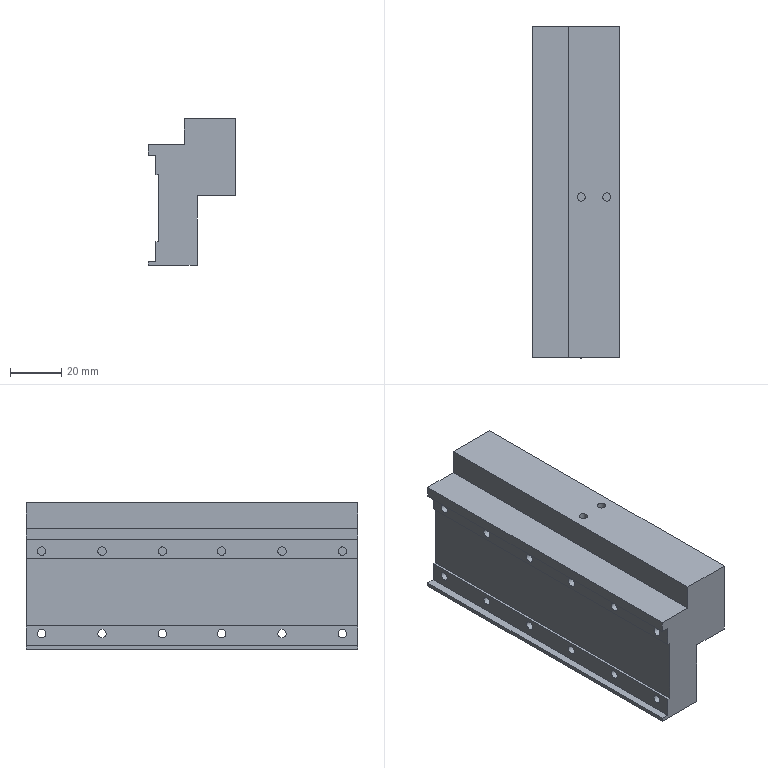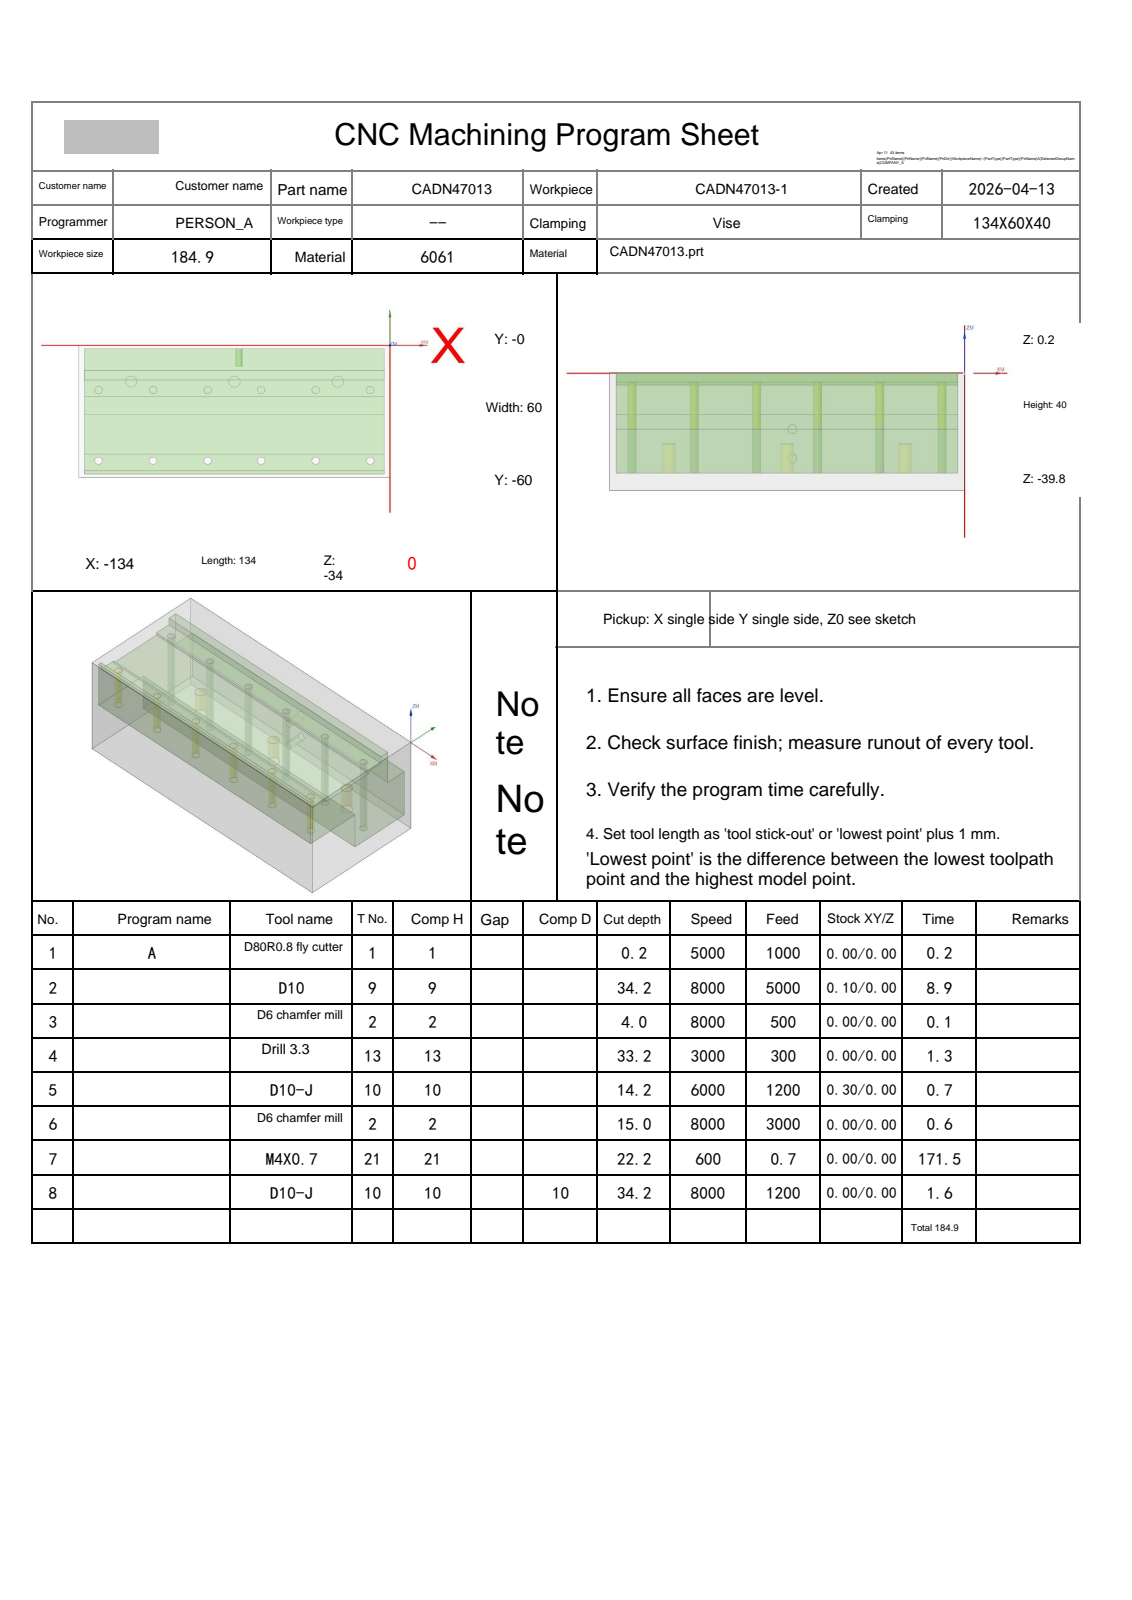NC program | NX | posted by the shop | part box 34 x 129 x 57 mm
Whole program:
%
O0001
(Machine time: 349.26 MIN)
(===Total Tool:6===)
(T1=D80R0.8 fly cutter D=80.  R=0.8  D-  H01 Z=-0.   )
(T9=D10     D=10.  R=0.   D-  H09 Z=-34.  )
(T2=D6 chamfer mill   D=6.   R=0.   D-  H02 Z=-14.8 )
(T13=Drill 3.3  D=3.3  DR_a=118 D-  H13 Z=-33.  )
(T10=D10-J  D=10.  R=0.   D-  H10 Z=-34.  )
(T21=M4X0.7 D=3.3  DR_a=180 D-  H21 Z=-22.  )
G80 G90 G17 G49 G40
G91 G28 Z0
M01
N1 T01 M06
(D80R0.8 fly cutter  D=80. R=0.8 H=01 ce=0.00 di=0.00)
G00 G90 G54 X42.5 Y-30. M03 S5000
G43 H01 Z20.
M08
Z2.
G01 Z0.0 F1000.
X37.5
X-171.5
X-176.5
Z2.
G00 Z20.
G91 G28 Z0.0
M05
M09
G91 G28 Z0.0
M01
N2 T09 M06
(D10  D=10. R=0. H=09 ce=0.10 di=0.00)
G00 G90 G54 X-67. Y3.6 M03 S8000
G43 H09 Z20.
M08
Z.5
G01 X-2.5 Z.375 F5000.
G02 X2.6 Y-1.5 Z.359 I0.0 J-5.1
G01 Y-58.5 Z.249
G02 X-2.5 Y-63.6 Z.233 I-5.1 J0.0
G01 X-131.5 Z-.017
G02 X-136.6 Y-58.5 Z-.033 I0.0 J5.1
G01 Y-1.5 Z-.143
G02 X-131.5 Y3.6 Z-.159 I5.1 J0.0
G01 X-2.5 Z-.409
G02 X2.6 Y-1.5 Z-.425 I0.0 J-5.1
G01 Y-58.5 Z-.535
G02 X-2.5 Y-63.6 Z-.551 I-5.1 J0.0
G01 X-131.5 Z-.801
G02 X-136.6 Y-58.5 Z-.817 I0.0 J5.1
G01 Y-1.5 Z-.927
G02 X-131.5 Y3.6 Z-.943 I5.1 J0.0
G01 X-2.5 Z-1.193
G02 X2.6 Y-1.5 Z-1.209 I0.0 J-5.1
G01 Y-58.5 Z-1.32
G02 X-2.5 Y-63.6 Z-1.335 I-5.1 J0.0
G01 X-131.5 Z-1.585
G02 X-136.6 Y-58.5 Z-1.601 I0.0 J5.1
G01 Y-1.5 Z-1.712
G02 X-131.5 Y3.6 Z-1.727 I5.1 J0.0
G01 X-2.5 Z-1.977
G02 X2.6 Y-1.5 Z-1.993 I0.0 J-5.1
G01 Y-58.5 Z-2.104
G02 X-2.5 Y-63.6 Z-2.119 I-5.1 J0.0
G01 X-131.5 Z-2.369
G02 X-136.6 Y-58.5 Z-2.385 I0.0 J5.1
G01 Y-1.5 Z-2.496
G02 X-131.5 Y3.6 Z-2.511 I5.1 J0.0
G01 X-2.5 Z-2.762
G02 X2.6 Y-1.5 Z-2.777 I0.0 J-5.1
G01 Y-58.5 Z-2.888
G02 X-2.5 Y-63.6 Z-2.903 I-5.1 J0.0
G01 X-131.5 Z-3.154
G02 X-136.6 Y-58.5 Z-3.169 I0.0 J5.1
G01 Y-1.5 Z-3.28
G02 X-131.5 Y3.6 Z-3.295 I5.1 J0.0
G01 X-2.5 Z-3.546
G02 X2.6 Y-1.5 Z-3.561 I0.0 J-5.1
G01 Y-58.5 Z-3.672
G02 X-2.5 Y-63.6 Z-3.687 I-5.1 J0.0
G01 X-131.5 Z-3.938
G02 X-136.6 Y-58.5 Z-3.953 I0.0 J5.1
G01 Y-1.5 Z-4.064
G02 X-131.5 Y3.6 Z-4.079 I5.1 J0.0
G01 X-2.5 Z-4.33
G02 X2.6 Y-1.5 Z-4.345 I0.0 J-5.1
G01 Y-58.5 Z-4.456
G02 X-2.5 Y-63.6 Z-4.471 I-5.1 J0.0
G01 X-131.5 Z-4.722
G02 X-136.6 Y-58.5 Z-4.737 I0.0 J5.1
G01 Y-1.5 Z-4.848
G02 X-131.5 Y3.6 Z-4.863 I5.1 J0.0
G01 X-2.5 Z-5.114
G02 X2.6 Y-1.5 Z-5.129 I0.0 J-5.1
G01 Y-58.5 Z-5.24
G02 X-2.5 Y-63.6 Z-5.256 I-5.1 J0.0
G01 X-131.5 Z-5.506
G02 X-136.6 Y-58.5 Z-5.521 I0.0 J5.1
G01 Y-1.5 Z-5.632
G02 X-131.5 Y3.6 Z-5.648 I5.1 J0.0
G01 X-2.5 Z-5.898
G02 X2.6 Y-1.5 Z-5.913 I0.0 J-5.1
G01 Y-58.5 Z-6.024
G02 X-2.5 Y-63.6 Z-6.04 I-5.1 J0.0
G01 X-131.5 Z-6.29
G02 X-136.6 Y-58.5 Z-6.305 I0.0 J5.1
G01 Y-1.5 Z-6.416
G02 X-131.5 Y3.6 Z-6.432 I5.1 J0.0
G01 X-2.5 Z-6.682
G02 X2.6 Y-1.5 Z-6.698 I0.0 J-5.1
G01 Y-58.5 Z-6.808
G02 X-2.5 Y-63.6 Z-6.824 I-5.1 J0.0
G01 X-131.5 Z-7.074
G02 X-136.6 Y-58.5 Z-7.09 I0.0 J5.1
G01 Y-1.5 Z-7.2
G02 X-131.5 Y3.6 Z-7.216 I5.1 J0.0
G01 X-2.5 Z-7.466
G02 X2.6 Y-1.5 Z-7.482 I0.0 J-5.1
G01 Y-58.5 Z-7.592
G02 X-2.5 Y-63.6 Z-7.608 I-5.1 J0.0
G01 X-131.5 Z-7.858
G02 X-136.6 Y-58.5 Z-7.874 I0.0 J5.1
G01 Y-1.5 Z-7.984
G02 X-131.5 Y3.6 Z-8. I5.1 J0.0
G01 X-2.5 Z-8.25
G02 X2.6 Y-1.5 Z-8.266 I0.0 J-5.1
G01 Y-58.5 Z-8.376
G02 X-2.5 Y-63.6 Z-8.392 I-5.1 J0.0
G01 X-131.5 Z-8.642
G02 X-136.6 Y-58.5 Z-8.658 I0.0 J5.1
G01 Y-1.5 Z-8.768
G02 X-131.5 Y3.6 Z-8.784 I5.1 J0.0
G01 X-2.5 Z-9.034
G02 X2.6 Y-1.5 Z-9.05 I0.0 J-5.1
G01 Y-58.5 Z-9.16
G02 X-2.5 Y-63.6 Z-9.176 I-5.1 J0.0
G01 X-131.5 Z-9.426
G02 X-136.6 Y-58.5 Z-9.442 I0.0 J5.1
G01 Y-1.5 Z-9.552
G02 X-131.5 Y3.6 Z-9.568 I5.1 J0.0
G01 X-2.5 Z-9.818
G02 X2.6 Y-1.5 Z-9.834 I0.0 J-5.1
G01 Y-58.5 Z-9.945
G02 X-2.5 Y-63.6 Z-9.96 I-5.1 J0.0
G01 X-131.5 Z-10.21
G02 X-136.6 Y-58.5 Z-10.226 I0.0 J5.1
G01 Y-1.5 Z-10.337
G02 X-131.5 Y3.6 Z-10.352 I5.1 J0.0
G01 X-2.5 Z-10.602
G02 X2.6 Y-1.5 Z-10.618 I0.0 J-5.1
G01 Y-58.5 Z-10.729
G02 X-2.5 Y-63.6 Z-10.744 I-5.1 J0.0
G01 X-131.5 Z-10.994
G02 X-136.6 Y-58.5 Z-11.01 I0.0 J5.1
G01 Y-1.5 Z-11.121
G02 X-131.5 Y3.6 Z-11.136 I5.1 J0.0
G01 X-2.5 Z-11.387
G02 X2.6 Y-1.5 Z-11.402 I0.0 J-5.1
G01 Y-58.5 Z-11.513
G02 X-2.5 Y-63.6 Z-11.528 I-5.1 J0.0
G01 X-131.5 Z-11.779
G02 X-136.6 Y-58.5 Z-11.794 I0.0 J5.1
G01 Y-1.5 Z-11.905
G02 X-131.5 Y3.6 Z-11.92 I5.1 J0.0
G01 X-2.5 Z-12.171
G02 X2.6 Y-1.5 Z-12.186 I0.0 J-5.1
G01 Y-58.5 Z-12.297
G02 X-2.5 Y-63.6 Z-12.312 I-5.1 J0.0
G01 X-131.5 Z-12.563
G02 X-136.6 Y-58.5 Z-12.578 I0.0 J5.1
G01 Y-1.5 Z-12.689
G02 X-131.5 Y3.6 Z-12.704 I5.1 J0.0
G01 X-2.5 Z-12.955
G02 X2.6 Y-1.5 Z-12.97 I0.0 J-5.1
G01 Y-58.5 Z-13.081
G02 X-2.5 Y-63.6 Z-13.096 I-5.1 J0.0
G01 X-131.5 Z-13.347
G02 X-136.6 Y-58.5 Z-13.362 I0.0 J5.1
G01 Y-1.5 Z-13.473
G02 X-131.5 Y3.6 Z-13.488 I5.1 J0.0
G01 X-2.5 Z-13.739
G02 X2.6 Y-1.5 Z-13.754 I0.0 J-5.1
G01 Y-58.5 Z-13.865
G02 X-2.5 Y-63.6 Z-13.881 I-5.1 J0.0
G01 X-131.5 Z-14.131
G02 X-136.6 Y-58.5 Z-14.146 I0.0 J5.1
G01 Y-1.5 Z-14.257
G02 X-131.5 Y3.6 Z-14.273 I5.1 J0.0
G01 X-2.5 Z-14.523
G02 X2.6 Y-1.5 Z-14.538 I0.0 J-5.1
G01 Y-58.5 Z-14.649
G02 X-2.5 Y-63.6 Z-14.665 I-5.1 J0.0
G01 X-131.5 Z-14.915
G02 X-136.6 Y-58.5 Z-14.93 I0.0 J5.1
G01 Y-1.5 Z-15.041
G02 X-131.5 Y3.6 Z-15.057 I5.1 J0.0
G01 X-2.5 Z-15.307
G02 X2.6 Y-1.5 Z-15.323 I0.0 J-5.1
G01 Y-58.5 Z-15.433
G02 X-2.5 Y-63.6 Z-15.449 I-5.1 J0.0
G01 X-131.5 Z-15.699
G02 X-136.6 Y-58.5 Z-15.715 I0.0 J5.1
G01 Y-1.5 Z-15.825
G02 X-131.5 Y3.6 Z-15.841 I5.1 J0.0
G01 X-2.5 Z-16.091
G02 X2.6 Y-1.5 Z-16.107 I0.0 J-5.1
G01 Y-58.5 Z-16.217
G02 X-2.5 Y-63.6 Z-16.233 I-5.1 J0.0
G01 X-131.5 Z-16.483
G02 X-136.6 Y-58.5 Z-16.499 I0.0 J5.1
G01 Y-1.5 Z-16.609
G02 X-131.5 Y3.6 Z-16.625 I5.1 J0.0
G01 X-2.5 Z-16.875
G02 X2.6 Y-1.5 Z-16.891 I0.0 J-5.1
G01 Y-58.5 Z-17.001
G02 X-2.5 Y-63.6 Z-17.017 I-5.1 J0.0
G01 X-131.5 Z-17.267
G02 X-136.6 Y-58.5 Z-17.283 I0.0 J5.1
G01 Y-1.5 Z-17.393
G02 X-131.5 Y3.6 Z-17.409 I5.1 J0.0
G01 X-2.5 Z-17.659
G02 X2.6 Y-1.5 Z-17.675 I0.0 J-5.1
G01 Y-58.5 Z-17.785
G02 X-2.5 Y-63.6 Z-17.801 I-5.1 J0.0
G01 X-131.5 Z-18.051
G02 X-136.6 Y-58.5 Z-18.067 I0.0 J5.1
G01 Y-1.5 Z-18.177
G02 X-131.5 Y3.6 Z-18.193 I5.1 J0.0
G01 X-2.5 Z-18.443
G02 X2.6 Y-1.5 Z-18.459 I0.0 J-5.1
G01 Y-58.5 Z-18.57
G02 X-2.5 Y-63.6 Z-18.585 I-5.1 J0.0
G01 X-131.5 Z-18.835
G02 X-136.6 Y-58.5 Z-18.851 I0.0 J5.1
G01 Y-1.5 Z-18.962
G02 X-131.5 Y3.6 Z-18.977 I5.1 J0.0
G01 X-2.5 Z-19.227
G02 X2.6 Y-1.5 Z-19.243 I0.0 J-5.1
G01 Y-58.5 Z-19.354
G02 X-2.5 Y-63.6 Z-19.369 I-5.1 J0.0
G01 X-131.5 Z-19.619
G02 X-136.6 Y-58.5 Z-19.635 I0.0 J5.1
G01 Y-1.5 Z-19.746
G02 X-131.5 Y3.6 Z-19.761 I5.1 J0.0
G01 X-2.5 Z-20.012
G02 X2.6 Y-1.5 Z-20.027 I0.0 J-5.1
G01 Y-58.5 Z-20.138
G02 X-2.5 Y-63.6 Z-20.153 I-5.1 J0.0
G01 X-131.5 Z-20.404
G02 X-136.6 Y-58.5 Z-20.419 I0.0 J5.1
G01 Y-1.5 Z-20.53
G02 X-131.5 Y3.6 Z-20.545 I5.1 J0.0
G01 X-2.5 Z-20.796
G02 X2.6 Y-1.5 Z-20.811 I0.0 J-5.1
G01 Y-58.5 Z-20.922
G02 X-2.5 Y-63.6 Z-20.937 I-5.1 J0.0
G01 X-131.5 Z-21.188
G02 X-136.6 Y-58.5 Z-21.203 I0.0 J5.1
G01 Y-1.5 Z-21.314
G02 X-131.5 Y3.6 Z-21.329 I5.1 J0.0
G01 X-2.5 Z-21.58
G02 X2.6 Y-1.5 Z-21.595 I0.0 J-5.1
G01 Y-58.5 Z-21.706
G02 X-2.5 Y-63.6 Z-21.721 I-5.1 J0.0
G01 X-131.5 Z-21.972
G02 X-136.6 Y-58.5 Z-21.987 I0.0 J5.1
G01 Y-1.5 Z-22.098
G02 X-131.5 Y3.6 Z-22.113 I5.1 J0.0
G01 X-2.5 Z-22.364
G02 X2.6 Y-1.5 Z-22.379 I0.0 J-5.1
G01 Y-58.5 Z-22.49
G02 X-2.5 Y-63.6 Z-22.506 I-5.1 J0.0
G01 X-131.5 Z-22.756
G02 X-136.6 Y-58.5 Z-22.771 I0.0 J5.1
G01 Y-1.5 Z-22.882
G02 X-131.5 Y3.6 Z-22.898 I5.1 J0.0
G01 X-2.5 Z-23.148
G02 X2.6 Y-1.5 Z-23.163 I0.0 J-5.1
G01 Y-58.5 Z-23.274
G02 X-2.5 Y-63.6 Z-23.29 I-5.1 J0.0
G01 X-131.5 Z-23.54
G02 X-136.6 Y-58.5 Z-23.555 I0.0 J5.1
G01 Y-1.5 Z-23.666
G02 X-131.5 Y3.6 Z-23.682 I5.1 J0.0
G01 X-2.5 Z-23.932
G02 X2.6 Y-1.5 Z-23.948 I0.0 J-5.1
G01 Y-58.5 Z-24.058
G02 X-2.5 Y-63.6 Z-24.074 I-5.1 J0.0
G01 X-131.5 Z-24.324
G02 X-136.6 Y-58.5 Z-24.34 I0.0 J5.1
G01 Y-1.5 Z-24.45
G02 X-131.5 Y3.6 Z-24.466 I5.1 J0.0
G01 X-2.5 Z-24.716
G02 X2.6 Y-1.5 Z-24.732 I0.0 J-5.1
G01 Y-58.5 Z-24.842
G02 X-2.5 Y-63.6 Z-24.858 I-5.1 J0.0
G01 X-131.5 Z-25.108
G02 X-136.6 Y-58.5 Z-25.124 I0.0 J5.1
G01 Y-1.5 Z-25.234
G02 X-131.5 Y3.6 Z-25.25 I5.1 J0.0
G01 X-2.5 Z-25.5
G02 X2.6 Y-1.5 Z-25.516 I0.0 J-5.1
G01 Y-58.5 Z-25.626
G02 X-2.5 Y-63.6 Z-25.642 I-5.1 J0.0
G01 X-131.5 Z-25.892
G02 X-136.6 Y-58.5 Z-25.908 I0.0 J5.1
G01 Y-1.5 Z-26.018
G02 X-131.5 Y3.6 Z-26.034 I5.1 J0.0
G01 X-2.5 Z-26.284
G02 X2.6 Y-1.5 Z-26.3 I0.0 J-5.1
G01 Y-58.5 Z-26.41
G02 X-2.5 Y-63.6 Z-26.426 I-5.1 J0.0
G01 X-131.5 Z-26.676
G02 X-136.6 Y-58.5 Z-26.692 I0.0 J5.1
G01 Y-1.5 Z-26.802
G02 X-131.5 Y3.6 Z-26.818 I5.1 J0.0
G01 X-2.5 Z-27.068
G02 X2.6 Y-1.5 Z-27.084 I0.0 J-5.1
G01 Y-58.5 Z-27.195
G02 X-2.5 Y-63.6 Z-27.21 I-5.1 J0.0
G01 X-131.5 Z-27.46
G02 X-136.6 Y-58.5 Z-27.476 I0.0 J5.1
G01 Y-1.5 Z-27.587
G02 X-131.5 Y3.6 Z-27.602 I5.1 J0.0
G01 X-2.5 Z-27.852
G02 X2.6 Y-1.5 Z-27.868 I0.0 J-5.1
G01 Y-58.5 Z-27.979
G02 X-2.5 Y-63.6 Z-27.994 I-5.1 J0.0
G01 X-131.5 Z-28.244
G02 X-136.6 Y-58.5 Z-28.26 I0.0 J5.1
G01 Y-1.5 Z-28.371
G02 X-131.5 Y3.6 Z-28.386 I5.1 J0.0
G01 X-2.5 Z-28.637
G02 X2.6 Y-1.5 Z-28.652 I0.0 J-5.1
G01 Y-58.5 Z-28.763
G02 X-2.5 Y-63.6 Z-28.778 I-5.1 J0.0
G01 X-131.5 Z-29.029
G02 X-136.6 Y-58.5 Z-29.044 I0.0 J5.1
G01 Y-1.5 Z-29.155
G02 X-131.5 Y3.6 Z-29.17 I5.1 J0.0
G01 X-2.5 Z-29.421
G02 X2.6 Y-1.5 Z-29.436 I0.0 J-5.1
G01 Y-58.5 Z-29.547
G02 X-2.5 Y-63.6 Z-29.562 I-5.1 J0.0
G01 X-131.5 Z-29.813
G02 X-136.6 Y-58.5 Z-29.828 I0.0 J5.1
G01 Y-1.5 Z-29.939
G02 X-131.5 Y3.6 Z-29.954 I5.1 J0.0
G01 X-2.5 Z-30.205
G02 X2.6 Y-1.5 Z-30.22 I0.0 J-5.1
G01 Y-58.5 Z-30.331
G02 X-2.5 Y-63.6 Z-30.346 I-5.1 J0.0
G01 X-131.5 Z-30.597
G02 X-136.6 Y-58.5 Z-30.612 I0.0 J5.1
G01 Y-1.5 Z-30.723
G02 X-131.5 Y3.6 Z-30.738 I5.1 J0.0
G01 X-2.5 Z-30.989
G02 X2.6 Y-1.5 Z-31.004 I0.0 J-5.1
G01 Y-58.5 Z-31.115
G02 X-2.5 Y-63.6 Z-31.131 I-5.1 J0.0
G01 X-131.5 Z-31.381
G02 X-136.6 Y-58.5 Z-31.396 I0.0 J5.1
G01 Y-1.5 Z-31.507
G02 X-131.5 Y3.6 Z-31.523 I5.1 J0.0
G01 X-2.5 Z-31.773
G02 X2.6 Y-1.5 Z-31.788 I0.0 J-5.1
G01 Y-58.5 Z-31.899
G02 X-2.5 Y-63.6 Z-31.915 I-5.1 J0.0
G01 X-131.5 Z-32.165
G02 X-136.6 Y-58.5 Z-32.18 I0.0 J5.1
G01 Y-1.5 Z-32.291
G02 X-131.5 Y3.6 Z-32.307 I5.1 J0.0
G01 X-2.5 Z-32.557
G02 X2.6 Y-1.5 Z-32.573 I0.0 J-5.1
G01 Y-58.5 Z-32.683
G02 X-2.5 Y-63.6 Z-32.699 I-5.1 J0.0
G01 X-131.5 Z-32.949
G02 X-136.6 Y-58.5 Z-32.965 I0.0 J5.1
G01 Y-1.5 Z-33.075
G02 X-131.5 Y3.6 Z-33.091 I5.1 J0.0
G01 X-2.5 Z-33.341
G02 X2.6 Y-1.5 Z-33.357 I0.0 J-5.1
G01 Y-58.5 Z-33.467
G02 X-2.5 Y-63.6 Z-33.483 I-5.1 J0.0
G01 X-131.5 Z-33.733
G02 X-136.6 Y-58.5 Z-33.749 I0.0 J5.1
G01 Y-1.5 Z-33.859
G02 X-131.5 Y3.6 Z-33.875 I5.1 J0.0
G01 X-67. Z-34.
X-2.5
G02 X2.6 Y-1.5 I0.0 J-5.1
G01 Y-58.5
G02 X-2.5 Y-63.6 I-5.1 J0.0
G01 X-131.5
G02 X-136.6 Y-58.5 I0.0 J5.1
G01 Y-1.5
G02 X-131.5 Y3.6 I5.1 J0.0
G01 X-67.
X-66.5
Z-33.
G00 Z20.
G00 G90 X-67. Y6.5 M03 S6000
Z20.
Z.004
G01 Z-.496 F3500.
Y-.5
X-132.5
Y-6.4
X-1.5
Y-.5
X-67.
X-67.5
Z.004
G00 Z.5
X-67. Y6.5
Z-.493
G01 Z-.993
Y-.5
X-132.5
Y-6.4
X-1.5
Y-.5
X-67.
X-67.5
Z-.493
G00 Z.004
X-67. Y6.5
Z-.989
G01 Z-1.489
Y-.5
X-132.5
Y-6.4
X-1.5
Y-.5
X-67.
X-67.5
Z-.989
G00 Z-.493
X-67. Y6.5
Z-1.486
G01 Z-1.986
Y-.5
X-132.5
Y-6.4
X-1.5
Y-.5
X-67.
X-67.5
Z-1.486
G00 Z-.989
X-67. Y6.5
Z-1.982
G01 Z-2.482
Y-.5
X-132.5
Y-6.4
X-1.5
Y-.5
X-67.
X-67.5
Z-1.982
G00 Z-1.486
X-67. Y6.5
Z-2.479
G01 Z-2.979
Y-.5
X-132.5
Y-6.4
X-1.5
Y-.5
X-67.
X-67.5
Z-2.479
G00 Z-1.982
X-67. Y6.5
Z-2.975
G01 Z-3.475
Y-.5
X-132.5
Y-6.4
X-1.5
Y-.5
X-67.
X-67.5
Z-2.975
G00 Z-2.479
X-67. Y6.5
Z-3.471
G01 Z-3.971
Y-.5
X-132.5
Y-6.4
X-1.5
Y-.5
X-67.
X-67.5
Z-3.471
G00 Z-2.975
X-67. Y6.5
Z-3.968
G01 Z-4.468
Y-.5
X-132.5
Y-6.4
X-1.5
Y-.5
X-67.
X-67.5
Z-3.968
G00 Z-3.471
X-67. Y6.5
Z-4.464
G01 Z-4.964
Y-.5
X-132.5
Y-6.4
X-1.5
Y-.5
X-67.
X-67.5
Z-4.464
G00 Z-3.968
X-67. Y6.5
Z-4.961
G01 Z-5.461
Y-.5
X-132.5
Y-6.4
X-1.5
Y-.5
X-67.
X-67.5
Z-4.961
G00 Z-4.464
X-67. Y6.5
Z-5.457
G01 Z-5.957
Y-.5
X-132.5
Y-6.4
X-1.5
Y-.5
X-67.
X-67.5
Z-5.457
G00 Z-4.961
X-67. Y6.5
Z-5.954
G01 Z-6.454
Y-.5
X-132.5
Y-6.4
X-1.5
Y-.5
X-67.
X-67.5
Z-5.954
G00 Z-5.457
X-67. Y6.5
Z-6.45
G01 Z-6.95
Y-.5
X-132.5
Y-6.4
X-1.5
Y-.5
X-67.
X-67.5
Z-6.45
G00 Z-5.954
X-67. Y6.5
Z-6.946
G01 Z-7.446
Y-.5
X-132.5
Y-6.4
X-1.5
Y-.5
X-67.
X-67.5
Z-6.946
G00 Z-6.45
X-67. Y6.5
Z-7.443
G01 Z-7.943
Y-.5
X-132.5
Y-6.4
X-1.5
Y-.5
X-67.
X-67.5
Z-7.443
G00 Z-6.946
X-67. Y6.5
Z-7.939
G01 Z-8.439
Y-.5
X-132.5
Y-6.4
X-1.5
Y-.5
X-67.
X-67.5
Z-7.939
G00 Z-7.443
X-67. Y6.5
Z-8.436
G01 Z-8.936
Y-.5
X-132.5
Y-6.4
X-1.5
Y-.5
X-67.
X-67.5
Z-8.436
G00 Z-7.939
X-67. Y6.5
Z-8.932
G01 Z-9.432
Y-.5
X-132.5
Y-6.4
X-1.5
Y-.5
X-67.
X-67.5
Z-8.932
G00 Z-8.436
X-67. Y6.5
Z-9.429
G01 Z-9.929
Y-.5
X-132.5
Y-6.4
X-1.5
Y-.5
X-67.
X-67.5
Z-9.429
G00 Z-8.932
X-67. Y6.5
Z-9.925
G01 Z-10.425
Y-.5
X-132.5
Y-6.4
X-1.5
Y-.5
X-67.
X-67.5
Z-9.925
G00 Z-9.429
X-67. Y6.5
Z-10.421
G01 Z-10.921
Y-.5
X-132.5
Y-6.4
X-1.5
Y-.5
X-67.
X-67.5
Z-10.421
G00 Z-9.925
X-67. Y6.5
Z-10.918
G01 Z-11.418
Y-.5
X-132.5
Y-6.4
X-1.5
Y-.5
X-67.
X-67.5
Z-10.918
G00 Z-10.421
X-67. Y6.5
Z-11.414
G01 Z-11.914
Y-.5
X-132.5
Y-6.4
X-1.5
Y-.5
X-67.
X-67.5
Z-11.414
G00 Z-10.918
X-67. Y6.5
Z-11.911
G01 Z-12.411
Y-.5
X-132.5
Y-6.4
X-1.5
Y-.5
X-67.
X-67.5
Z-11.911
G00 Z-11.414
X-67. Y6.5
Z-12.407
G01 Z-12.907
Y-.5
X-132.5
Y-6.4
X-1.5
Y-.5
X-67.
X-67.5
Z-12.407
G00 Z-11.911
X-67. Y6.5
Z-12.904
G01 Z-13.404
Y-.5
X-132.5
Y-6.4
X-1.5
Y-.5
X-67.
X-67.5
Z-12.904
G00 Z-12.407
X-67. Y6.5
Z-13.4
G01 Z-13.9
Y-.5
X-132.5
Y-6.4
X-1.5
Y-.5
X-67.
X-67.5
Z-13.4
G00 Z20.
G00 G90 X-139.5 Y-36.377 M03 S6000
Z20.
Z.013
G01 Z-.488 F3500.
X-132.5
Y-28.427
X-1.5
Y-44.327
X-132.5
Y-36.377
X-125.5
Y-35.427
X-8.5
Y-37.327
X-125.5
Y-36.377
Y-35.877
Z.013
G00 Z.5
X-139.5 Y-36.377
Z-.475
G01 Z-.975
X-132.5
Y-28.427
X-1.5
Y-44.327
X-132.5
Y-36.377
X-125.5
Y-35.427
X-8.5
Y-37.327
X-125.5
Y-36.377
Y-35.877
Z-.475
G00 Z.013
X-139.5 Y-36.377
Z-.963
G01 Z-1.463
X-132.5
Y-28.427
X-1.5
Y-44.327
X-132.5
Y-36.377
X-125.5
Y-35.427
X-8.5
Y-37.327
X-125.5
Y-36.377
Y-35.877
Z-.963
G00 Z-.475
X-139.5 Y-36.377
Z-1.45
G01 Z-1.95
X-132.5
Y-28.427
X-1.5
Y-44.327
X-132.5
Y-36.377
X-125.5
Y-35.427
X-8.5
Y-37.327
X-125.5
Y-36.377
Y-35.877
Z-1.45
G00 Z-.963
X-139.5 Y-36.377
Z-1.938
G01 Z-2.438
X-132.5
Y-28.427
X-1.5
Y-44.327
X-132.5
Y-36.377
X-125.5
Y-35.427
X-8.5
Y-37.327
X-125.5
Y-36.377
Y-35.877
Z-1.938
G00 Z-1.45
X-139.5 Y-36.377
Z-2.425
G01 Z-2.925
X-132.5
Y-28.427
X-1.5
Y-44.327
X-132.5
Y-36.377
X-125.5
Y-35.427
X-8.5
Y-37.327
X-125.5
Y-36.377
Y-35.877
Z-2.425
G00 Z-1.938
X-139.5 Y-36.377
Z-2.913
G01 Z-3.413
X-132.5
Y-28.427
X-1.5
Y-44.327
X-132.5
Y-36.377
X-125.5
Y-35.427
X-8.5
Y-37.327
X-125.5
Y-36.377
Y-35.877
Z-2.913
G00 Z-2.425
X-139.5 Y-36.377
Z-3.4
G01 Z-3.9
X-132.5
Y-28.427
X-1.5
Y-44.327
X-132.5
Y-36.377
X-125.5
Y-35.427
X-8.5
Y-37.327
X-125.5
Y-36.377
Y-35.877
Z-3.4
G00 Z20.
G00 G90 X-67. Y-31.327 M03 S6000
Z20.
Z.258
G01 Z-.242 F4000.
Y-24.327
X-1.5
Y-20.827
X-132.5
Y-24.327
X-67.
X-66.5
Z.258
G00 Z.5
X-67. Y-31.327
Z.017
G01 Z-.483
Y-24.327
X-1.5
Y-20.827
X-132.5
Y-24.327
X-67.
X-66.5
Z.017
G00 Z.258
X-67. Y-31.327
Z-.225
G01 Z-.725
Y-24.327
X-1.5
Y-20.827
X-132.5
Y-24.327
X-67.
X-66.5
Z-.225
G00 Z.017
X-67. Y-31.327
Z-.467
G01 Z-.967
Y-24.327
X-1.5
Y-20.827
X-132.5
Y-24.327
X-67.
X-66.5
Z-.467
G00 Z-.225
X-67. Y-31.327
Z-.708
G01 Z-1.208
Y-24.327
X-1.5
Y-20.827
X-132.5
Y-24.327
X-67.
X-66.5
Z-.708
G00 Z-.467
X-67. Y-31.327
Z-.95
G01 Z-1.45
Y-24.327
X-1.5
Y-20.827
X-132.5
Y-24.327
X-67.
X-66.5
Z-.95
G00 Z-.708
X-67. Y-31.327
Z-1.192
G01 Z-1.692
Y-24.327
X-1.5
Y-20.827
X-132.5
Y-24.327
X-67.
X-66.5
Z-1.192
G00 Z-.95
X-67. Y-31.327
Z-1.433
G01 Z-1.933
Y-24.327
X-1.5
Y-20.827
X-132.5
Y-24.327
X-67.
X-66.5
Z-1.433
G00 Z-1.192
X-67. Y-31.327
Z-1.675
G01 Z-2.175
Y-24.327
X-1.5
Y-20.827
X-132.5
Y-24.327
X-67.
X-66.5
Z-1.675
G00 Z-1.433
X-67. Y-31.327
Z-1.917
G01 Z-2.417
Y-24.327
X-1.5
Y-20.827
X-132.5
Y-24.327
X-67.
X-66.5
Z-1.917
G00 Z-1.675
X-67. Y-31.327
Z-2.158
G01 Z-2.658
Y-24.327
X-1.5
Y-20.827
X-132.5
Y-24.327
X-67.
X-66.5
Z-2.158
G00 Z-1.917
X-67. Y-31.327
Z-2.4
G01 Z-2.9
Y-24.327
X-1.5
Y-20.827
X-132.5
Y-24.327
X-67.
X-66.5
Z-2.4
G00 Z20.
X-67. Y-41.427
Z.258
G01 Z-.242
Y-48.427
X-132.5
Y-51.927
X-1.5
Y-48.427
X-67.
X-67.5
Z.258
G00 Z.5
X-67. Y-41.427
Z.017
G01 Z-.483
Y-48.427
X-132.5
Y-51.927
X-1.5
Y-48.427
X-67.
X-67.5
Z.017
G00 Z.258
X-67. Y-41.427
Z-.225
G01 Z-.725
Y-48.427
X-132.5
Y-51.927
X-1.5
Y-48.427
X-67.
X-67.5
Z-.225
G00 Z.017
X-67. Y-41.427
Z-.467
G01 Z-.967
Y-48.427
X-132.5
Y-51.927
X-1.5
Y-48.427
X-67.
X-67.5
Z-.467
G00 Z-.225
X-67. Y-41.427
Z-.708
G01 Z-1.208
Y-48.427
X-132.5
Y-51.927
X-1.5
Y-48.427
X-67.
X-67.5
Z-.708
G00 Z-.467
X-67. Y-41.427
Z-.95
G01 Z-1.45
Y-48.427
X-132.5
Y-51.927
X-1.5
Y-48.427
X-67.
X-67.5
Z-.95
G00 Z-.708
X-67. Y-41.427
Z-1.192
G01 Z-1.692
Y-48.427
X-132.5
Y-51.927
X-1.5
Y-48.427
X-67.
X-67.5
Z-1.192
G00 Z-.95
X-67. Y-41.427
Z-1.433
G01 Z-1.933
Y-48.427
X-132.5
Y-51.927
X-1.5
Y-48.427
X-67.
X-67.5
Z-1.433
G00 Z-1.192
X-67. Y-41.427
Z-1.675
G01 Z-2.175
Y-48.427
X-132.5
Y-51.927
X-1.5
Y-48.427
X-67.
X-67.5
Z-1.675
G00 Z-1.433
X-67. Y-41.427
Z-1.917
G01 Z-2.417
Y-48.427
X-132.5
Y-51.927
X-1.5
Y-48.427
X-67.
X-67.5
Z-1.917
G00 Z-1.675
X-67. Y-41.427
Z-2.158
G01 Z-2.658
Y-48.427
X-132.5
Y-51.927
X-1.5
Y-48.427
X-67.
X-67.5
Z-2.158
G00 Z-1.917
X-67. Y-41.427
Z-2.4
G01 Z-2.9
Y-48.427
X-132.5
Y-51.927
X-1.5
Y-48.427
X-67.
X-67.5
Z-2.4
G00 Z20.
G91 G28 Z0.0
M05
M09
G91 G28 Z0.0
M01
N3 T02 M06
(D6 chamfer mill  D=6. R=0. H=02 ce=0.00 di=0.10)
G00 G90 G54 X-8.5 Y-52.427 M03 S8000
G43 H02 Z20.
M08
G98 G81 X-8.5 Y-52.427 Z-3.8 R-2. F500.
X-32.
X-55.5
X-78.5
X-102.
X-125.5
Y-20.327
X-102.
X-78.5
X-55.5
X-32.
X-8.5
G80
G00 Z20.
G91 G28 Z0.0
M05
M09
G91 G28 Z0.0
M01
N4 T13 M06
(Drill 3.3 D=3.3 DR_a=118 H=13)
G00 G90 G54 X-125.5 Y-52.427 M03 S3000
G43 H13 Z20.
M08
G98 G83 X-125.5 Y-52.427 Z-24.991 R-2. F300. Q2.
X-102.
X-78.5
X-55.5
X-32.
X-8.5
G80
G00 Z20.
G00 G90 X-125.5 Y-20.327 M03 S3000
Z20.
G98 G83 X-125.5 Y-20.327 Z-33. R-2. F250. Q2.
X-102.
X-78.5
X-55.5
X-32.
X-8.5
G80
G00 Z20.
G91 G28 Z0.0
M05
M09
G91 G28 Z0.0
M01
N5 T10 M06
(D10-J  D=10. R=0. H=10 ce=0.30 di=0.00)
G00 G90 G54 X-139.5 Y-.5 M03 S6000
G43 H10 Z20.
M08
Z-13.5
G01 Z-14. F1200.
X-136.5
X2.5
Y-6.2
X-136.5
X-139.8
Z-13.5
G00 Z20.
G00 G90 X5.8 Y-44.126 M03 S6000
Z20.
Z-3.5
G01 Z-4. F1200.
X2.5
X-136.5
Y-38.96
X2.5
Y-33.793
X-136.5
Y-28.627
X2.5
X5.8
Z-3.5
G00 Z20.
G91 G28 Z0.0
M05
M09
G91 G28 Z0.0
M01
N6 T02 M06
(D6 chamfer mill  D=6. R=0. H=02 ce=0.00 di=0.00)
G00 G90 G54 X-66.75 Y-59.928 M03 S8000
G43 H02 Z20.
M08
Z2.799
G01 Z-.799 F3000.
G03 X-66.67 Y-59.628 I-.52 J.3
X-66.97 Y-59.108 I-.6 J0.0
G01 X-67. Y-59.1
X-131.5
G02 X-132.1 Y-58.5 I0.0 J.6
G01 Y-57.027
G02 X-131.5 Y-56.427 I.6 J0.0
G01 X-2.5
G02 X-1.9 Y-57.027 I0.0 J-.6
G01 Y-58.5
G02 X-2.5 Y-59.1 I-.6 J0.0
G01 X-67.
X-67.03 Y-59.108
G03 X-67.33 Y-59.628 I.3 J-.52
X-67.25 Y-59.928 I.6 J0.0
G01 Z2.799
G00 Z20.
Y-10.072
Z2.799
G01 Z-.799
G03 X-67.33 Y-10.372 I.52 J-.3
X-67.03 Y-10.892 I.6 J0.0
G01 X-67. Y-10.9
X-2.5
G02 X-1.9 Y-11.5 I0.0 J-.6
G01 Y-15.727
G02 X-2.5 Y-16.327 I-.6 J0.0
G01 X-131.5
G02 X-132.1 Y-15.727 I0.0 J.6
G01 Y-11.5
G02 X-131.5 Y-10.9 I.6 J0.0
G01 X-67.
X-66.97 Y-10.892
G03 X-66.67 Y-10.372 I-.3 J.52
X-66.75 Y-10.072 I-.6 J0.0
G01 Z2.799
G00 Z20.
X-1.486 Y-19.076
Z2.455
G01 Z-3.799
X-1.636 Y-19.035
G03 X-1.896 Y-19.185 I0.0 J-.3
G01 X-1.9 Y-19.2
Y-23.327
G02 X-2.5 Y-23.927 I-.6 J0.0
G01 X-131.5
G02 X-132.1 Y-23.327 I0.0 J.6
G01 Y-19.2
X-132.104 Y-19.185
G03 X-132.364 Y-19.035 I-.26 J-.15
G01 X-132.514 Y-19.076
Z2.455
G00 Z20.
Y-53.678
Z2.455
G01 Z-3.799
X-132.364 Y-53.719
G03 X-132.104 Y-53.569 I0.0 J.3
G01 X-132.1 Y-53.554
Y-49.427
G02 X-131.5 Y-48.827 I.6 J0.0
G01 X-2.5
G02 X-1.9 Y-49.427 I0.0 J-.6
G01 Y-53.554
X-1.896 Y-53.569
G03 X-1.636 Y-53.719 I.26 J.15
G01 X-1.486 Y-53.678
Z2.455
G00 Z20.
X-132.1 Y-47.745
Z-.545
G01 Z-4.799
Y-25.009
Z-.545
G00 Z20.
X-1.9
Z-.545
G01 Z-4.799
Y-47.745
Z-.545
G00 Z20.
X-132.597 Y-8.173
Z2.455
G01 Z-14.799
X-132.417 Y-8.221
G03 X-132.105 Y-8.041 I0.0 J.36
G01 X-132.1 Y-8.023
Y-1.5
G02 X-131.5 Y-.9 I.6 J0.0
G01 X-2.5
G02 X-1.9 Y-1.5 I0.0 J-.6
G01 Y-8.023
X-1.895 Y-8.041
G03 X-1.583 Y-8.221 I.312 J.18
G01 X-1.403 Y-8.173
Z2.455
G00 Z20.
G00 G90 X-8.5 Y-52.427 M03 S8000
Z20.
G98 G81 X-8.5 Y-52.427 Z-5.2 R0.0 F500.
X-32.
X-55.5
X-78.5
X-102.
X-125.5
Y-20.327
X-102.
X-78.5
X-55.5
X-32.
X-8.5
G80
G00 Z20.
G91 G28 Z0.0
M05
M09
G91 G28 Z0.0
M01
N7 T21 M06
(M4X0.7 D=3.3 DR_a=180 H=21)
G00 G90 G54 X-125.5 Y-52.427 M03 S600
G43 H21 Z20.
M08
G95
G98 G84 X-125.5 Y-52.427 Z-22. R-2. F.7 Q4.
X-102.
X-78.5
X-55.5
X-32.
X-8.5
G80
G94
G00 Z20.
G91 G28 Z0.0
M05
M09
G91 G28 Z0.0
M01
N8 T10 M06
(D10-J  D=10. R=0. H=10 ce=0.00 di=0.01)
G00 G90 G54 X-137. Y-5.4 M03 S6000
G43 H10 Z20.
M08
Z-6.498
G01 Z-6.998 F1200.
G41 D10
Y-5.5
G03 X-136. Y-6.5 I1. J0.0
G01 X2.
G03 X3. Y-5.5 I0.0 J1.
G01 G40 Y-5.4
Z-6.498
G00 Z20.
X-137.
Z-13.495
G01 Z-13.995
G41 D10
Y-5.5
G03 X-136. Y-6.5 I1. J0.0
G01 X2.
G03 X3. Y-5.5 I0.0 J1.
G01 G40 Y-5.4
Z-13.495
G00 Z20.
G00 G90 X3. Y-29.427 M03 S6000
Z20.
Z-3.495
G01 Z-3.995 F1200.
G41 D10
Y-29.327
G03 X2. Y-28.327 I-1. J0.0
G01 X-136.
G03 X-137. Y-29.327 I0.0 J-1.
G01 G40 Y-29.427
Z-3.495
G00 Z20.
Y-43.327
Z-3.495
G01 Z-3.995
G41 D10
Y-43.427
G03 X-136. Y-44.427 I1. J0.0
G01 X2.
G03 X3. Y-43.427 I0.0 J1.
G01 G40 Y-43.327
Z-3.495
G00 Z20.
G00 G90 X-137. Y-50.927 M03 S6000
Z20.
Z-2.5
G01 Z-3. F1200.
G41 D10
Y-51.027
G03 X-136. Y-52.027 I1. J0.0
G01 X2.
G03 X3. Y-51.027 I0.0 J1.
G01 G40 Y-50.927
Z-2.5
G00 Z20.
Y-21.827
Z-2.5
G01 Z-3.
G41 D10
Y-21.727
G03 X2. Y-20.727 I-1. J0.0
G01 X-136.
G03 X-137. Y-21.727 I0.0 J-1.
G01 G40 Y-21.827
Z-2.5
G00 Z20.
G00 G90 X-1.487 Y-64.616 M03 S8000
Z20.
Z-16.5
G01 Z-17. F1000.
G41 D10
X-1.503 Y-64.417
G03 X-2.5 Y-63.5 I-.997 J-.083
G01 X-131.5
G02 X-136.5 Y-58.5 I0.0 J5.
G01 Y-1.5
G02 X-131.5 Y3.5 I5. J0.0
G01 X-2.5
G02 X2.5 Y-1.5 I0.0 J-5.
G01 Y-58.5
G02 X-2.5 Y-63.5 I-5. J0.0
G01 X-3.
G03 X-4. Y-64.5 I0.0 J-1.
G01 G40 Y-64.7
Z-16.5
G00 Z20.
X-1.487 Y-64.616
Z-33.5
G01 Z-34.
G41 D10
X-1.503 Y-64.417
G03 X-2.5 Y-63.5 I-.997 J-.083
G01 X-131.5
G02 X-136.5 Y-58.5 I0.0 J5.
G01 Y-1.5
G02 X-131.5 Y3.5 I5. J0.0
G01 X-2.5
G02 X2.5 Y-1.5 I0.0 J-5.
G01 Y-58.5
G02 X-2.5 Y-63.5 I-5. J0.0
G01 X-3.
G03 X-4. Y-64.5 I0.0 J-1.
G01 G40 Y-64.7
Z-33.5
G00 Z20.
M05
M09
G91 G28 Z0.0
G91 G28 Y0.0
M30
%